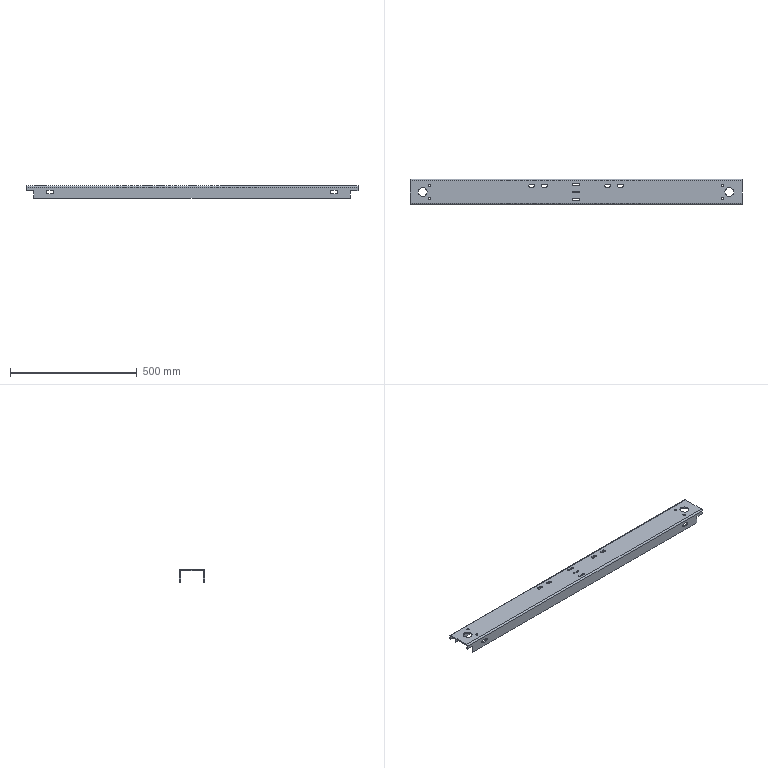Part | SolidWorks | features ICE 4, FlatPattern 1, MirrorPattern 1, SMBaseFlange 1, SheetMetal 1 | 1 solid | 93 faces | box 1310 x 100 x 50 mm | volume 1180927 mm3 | plane 48 | cylinder 45 | commonest cylinder face diameters 13 x20 7 x9 8.6 x8 35 x4 2 x2 12 x2